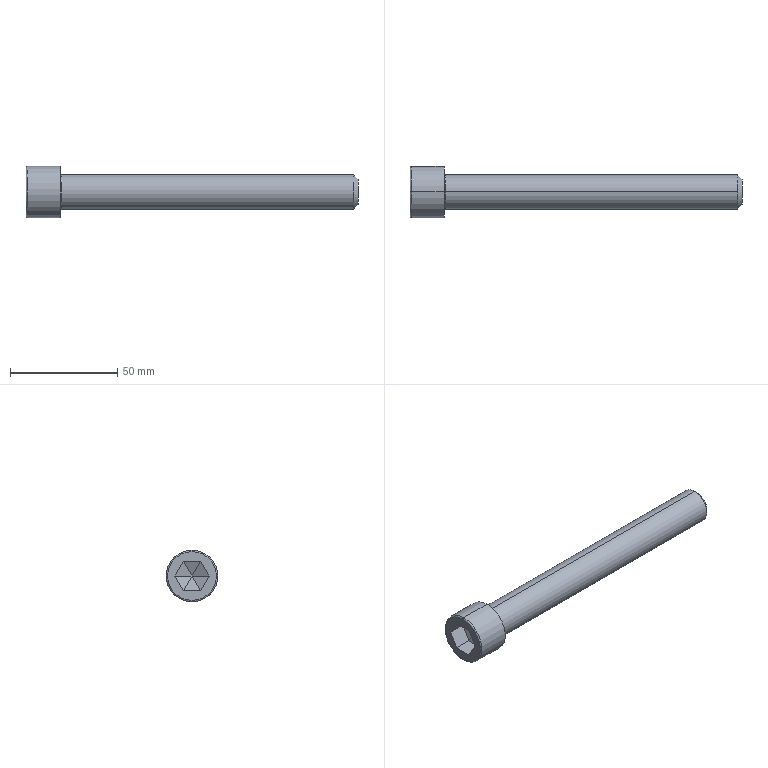Part | SolidWorks | features BlendCut 1, Chamfer 1, Cut 1, Fillet 1, ICE 1, LPattern 1, RevCut 1, Revolution 1 | 1 solid | 25 faces | box 155 x 24 x 24 mm | volume 33595 mm3 | plane 15 | torus 4 | cylinder 4 | cone 2 | commonest cylinder face diameters 16 x2 24 x2
STEP:
#1=CARTESIAN_POINT('',(155.,0.,-6.));
#2=VERTEX_POINT('',#1);
#3=CARTESIAN_POINT('',(155.,0.,6.));
#4=VERTEX_POINT('',#3);
#5=CARTESIAN_POINT('',(155.,0.,0.));
#6=DIRECTION('',(1.,0.,0.));
#7=DIRECTION('',(0.,0.,-1.));
#8=AXIS2_PLACEMENT_3D('',#5,#6,#7);
#9=CIRCLE('',#8,6.);
#10=EDGE_CURVE('',#2,#4,#9,.T.);
#11=ORIENTED_EDGE('',*,*,#10,.F.);
#12=CARTESIAN_POINT('',(153.,0.,-8.));
#13=VERTEX_POINT('',#12);
#14=CARTESIAN_POINT('',(155.,0.,-6.));
#15=DIRECTION('',(-0.7071,0.,-0.7071));
#16=VECTOR('',#15,1000.);
#17=LINE('',#14,#16);
#18=EDGE_CURVE('',#2,#13,#17,.T.);
#19=ORIENTED_EDGE('',*,*,#18,.T.);
#20=CARTESIAN_POINT('',(153.,0.,8.));
#21=VERTEX_POINT('',#20);
#22=CARTESIAN_POINT('',(153.,0.,0.));
#23=DIRECTION('',(-1.,0.,0.));
#24=DIRECTION('',(0.,0.,-1.));
#25=AXIS2_PLACEMENT_3D('',#22,#23,#24);
#26=CIRCLE('',#25,8.);
#27=EDGE_CURVE('',#21,#13,#26,.T.);
#28=ORIENTED_EDGE('',*,*,#27,.F.);
#29=CARTESIAN_POINT('',(155.,0.,6.));
#30=DIRECTION('',(-0.7071,0.,0.7071));
#31=VECTOR('',#30,1000.);
#32=LINE('',#29,#31);
#33=EDGE_CURVE('',#4,#21,#32,.T.);
#34=ORIENTED_EDGE('',*,*,#33,.F.);
#35=EDGE_LOOP('',(#11,#19,#28,#34));
#36=FACE_OUTER_BOUND('',#35,.T.);
#37=CARTESIAN_POINT('',(155.,0.,0.));
#38=DIRECTION('',(-1.,0.,0.));
#39=DIRECTION('',(0.,0.,1.));
#40=AXIS2_PLACEMENT_3D('',#37,#38,#39);
#41=CONICAL_SURFACE('',#40,6.,0.7854);
#42=ADVANCED_FACE('',(#36),#41,.T.);
#43=CARTESIAN_POINT('',(0.6,0.,-12.));
#44=VERTEX_POINT('',#43);
#45=CARTESIAN_POINT('',(0.6,0.,12.));
#46=VERTEX_POINT('',#45);
#47=CARTESIAN_POINT('',(0.6,0.,0.));
#48=DIRECTION('',(1.,0.,0.));
#49=DIRECTION('',(0.,0.,1.));
#50=AXIS2_PLACEMENT_3D('',#47,#48,#49);
#51=CIRCLE('',#50,12.);
#52=EDGE_CURVE('',#44,#46,#51,.T.);
#53=ORIENTED_EDGE('',*,*,#52,.F.);
#54=CARTESIAN_POINT('',(0.,0.,-11.4));
#55=VERTEX_POINT('',#54);
#56=CARTESIAN_POINT('',(0.6,0.,-11.4));
#57=DIRECTION('',(0.,1.,0.));
#58=DIRECTION('',(0.,0.,1.));
#59=AXIS2_PLACEMENT_3D('',#56,#57,#58);
#60=CIRCLE('',#59,0.6);
#61=EDGE_CURVE('',#44,#55,#60,.T.);
#62=ORIENTED_EDGE('',*,*,#61,.T.);
#63=CARTESIAN_POINT('',(0.,0.,11.4));
#64=VERTEX_POINT('',#63);
#65=CARTESIAN_POINT('',(0.,0.,0.));
#66=DIRECTION('',(-1.,0.,0.));
#67=DIRECTION('',(0.,0.,1.));
#68=AXIS2_PLACEMENT_3D('',#65,#66,#67);
#69=CIRCLE('',#68,11.4);
#70=EDGE_CURVE('',#64,#55,#69,.T.);
#71=ORIENTED_EDGE('',*,*,#70,.F.);
#72=CARTESIAN_POINT('',(0.6,0.,11.4));
#73=DIRECTION('',(0.,-1.,0.));
#74=DIRECTION('',(0.,0.,-1.));
#75=AXIS2_PLACEMENT_3D('',#72,#73,#74);
#76=CIRCLE('',#75,0.6);
#77=EDGE_CURVE('',#46,#64,#76,.T.);
#78=ORIENTED_EDGE('',*,*,#77,.F.);
#79=EDGE_LOOP('',(#53,#62,#71,#78));
#80=FACE_OUTER_BOUND('',#79,.T.);
#81=CARTESIAN_POINT('',(0.6,0.,0.));
#82=DIRECTION('',(-1.,0.,0.));
#83=DIRECTION('',(0.,0.,1.));
#84=AXIS2_PLACEMENT_3D('',#81,#82,#83);
#85=TOROIDAL_SURFACE('',#84,11.4,0.6);
#86=ADVANCED_FACE('',(#80),#85,.T.);
#87=CARTESIAN_POINT('',(16.6,0.,8.));
#88=VERTEX_POINT('',#87);
#89=CARTESIAN_POINT('',(16.6,0.,-8.));
#90=VERTEX_POINT('',#89);
#91=CARTESIAN_POINT('',(16.6,0.,0.));
#92=DIRECTION('',(1.,0.,0.));
#93=DIRECTION('',(0.,0.,-1.));
#94=AXIS2_PLACEMENT_3D('',#91,#92,#93);
#95=CIRCLE('',#94,8.);
#96=EDGE_CURVE('',#88,#90,#95,.T.);
#97=ORIENTED_EDGE('',*,*,#96,.F.);
#98=CARTESIAN_POINT('',(16.,0.,8.6));
#99=VERTEX_POINT('',#98);
#100=CARTESIAN_POINT('',(16.6,0.,8.6));
#101=DIRECTION('',(0.,1.,0.));
#102=DIRECTION('',(0.,0.,1.));
#103=AXIS2_PLACEMENT_3D('',#100,#101,#102);
#104=CIRCLE('',#103,0.6);
#105=EDGE_CURVE('',#88,#99,#104,.T.);
#106=ORIENTED_EDGE('',*,*,#105,.T.);
#107=CARTESIAN_POINT('',(16.,0.,-8.6));
#108=VERTEX_POINT('',#107);
#109=CARTESIAN_POINT('',(16.,0.,0.));
#110=DIRECTION('',(1.,0.,0.));
#111=DIRECTION('',(0.,0.,-1.));
#112=AXIS2_PLACEMENT_3D('',#109,#110,#111);
#113=CIRCLE('',#112,8.6);
#114=EDGE_CURVE('',#99,#108,#113,.T.);
#115=ORIENTED_EDGE('',*,*,#114,.T.);
#116=CARTESIAN_POINT('',(16.6,0.,-8.6));
#117=DIRECTION('',(0.,-1.,0.));
#118=DIRECTION('',(0.,0.,-1.));
#119=AXIS2_PLACEMENT_3D('',#116,#117,#118);
#120=CIRCLE('',#119,0.6);
#121=EDGE_CURVE('',#90,#108,#120,.T.);
#122=ORIENTED_EDGE('',*,*,#121,.F.);
#123=EDGE_LOOP('',(#97,#106,#115,#122));
#124=FACE_OUTER_BOUND('',#123,.T.);
#125=CARTESIAN_POINT('',(16.6,0.,0.));
#126=DIRECTION('',(1.,0.,0.));
#127=DIRECTION('',(0.,0.,-1.));
#128=AXIS2_PLACEMENT_3D('',#125,#126,#127);
#129=TOROIDAL_SURFACE('',#128,8.6,0.6);
#130=ADVANCED_FACE('',(#124),#129,.F.);
#131=ORIENTED_EDGE('',*,*,#52,.T.);
#132=CARTESIAN_POINT('',(16.,0.,12.));
#133=VERTEX_POINT('',#132);
#134=CARTESIAN_POINT('',(0.,0.,12.));
#135=DIRECTION('',(1.,0.,0.));
#136=VECTOR('',#135,1000.);
#137=LINE('',#134,#136);
#138=EDGE_CURVE('',#46,#133,#137,.T.);
#139=ORIENTED_EDGE('',*,*,#138,.T.);
#140=CARTESIAN_POINT('',(16.,0.,-12.));
#141=VERTEX_POINT('',#140);
#142=CARTESIAN_POINT('',(16.,0.,0.));
#143=DIRECTION('',(1.,0.,0.));
#144=DIRECTION('',(0.,0.,-1.));
#145=AXIS2_PLACEMENT_3D('',#142,#143,#144);
#146=CIRCLE('',#145,12.);
#147=EDGE_CURVE('',#141,#133,#146,.T.);
#148=ORIENTED_EDGE('',*,*,#147,.F.);
#149=CARTESIAN_POINT('',(0.,0.,-12.));
#150=DIRECTION('',(1.,0.,0.));
#151=VECTOR('',#150,1000.);
#152=LINE('',#149,#151);
#153=EDGE_CURVE('',#44,#141,#152,.T.);
#154=ORIENTED_EDGE('',*,*,#153,.F.);
#155=EDGE_LOOP('',(#131,#139,#148,#154));
#156=FACE_OUTER_BOUND('',#155,.T.);
#157=CARTESIAN_POINT('',(0.,0.,0.));
#158=DIRECTION('',(1.,0.,0.));
#159=DIRECTION('',(0.,0.,-1.));
#160=AXIS2_PLACEMENT_3D('',#157,#158,#159);
#161=CYLINDRICAL_SURFACE('',#160,12.);
#162=ADVANCED_FACE('',(#156),#161,.T.);
#163=CARTESIAN_POINT('',(16.6,0.,0.));
#164=DIRECTION('',(1.,0.,0.));
#165=DIRECTION('',(0.,0.,-1.));
#166=AXIS2_PLACEMENT_3D('',#163,#164,#165);
#167=CIRCLE('',#166,8.);
#168=EDGE_CURVE('',#90,#88,#167,.T.);
#169=ORIENTED_EDGE('',*,*,#168,.T.);
#170=CARTESIAN_POINT('',(0.,0.,8.));
#171=DIRECTION('',(1.,0.,0.));
#172=VECTOR('',#171,1000.);
#173=LINE('',#170,#172);
#174=EDGE_CURVE('',#88,#21,#173,.T.);
#175=ORIENTED_EDGE('',*,*,#174,.T.);
#176=ORIENTED_EDGE('',*,*,#27,.T.);
#177=CARTESIAN_POINT('',(0.,0.,-8.));
#178=DIRECTION('',(1.,0.,0.));
#179=VECTOR('',#178,1000.);
#180=LINE('',#177,#179);
#181=EDGE_CURVE('',#90,#13,#180,.T.);
#182=ORIENTED_EDGE('',*,*,#181,.F.);
#183=EDGE_LOOP('',(#169,#175,#176,#182));
#184=FACE_OUTER_BOUND('',#183,.T.);
#185=CARTESIAN_POINT('',(0.,0.,0.));
#186=DIRECTION('',(1.,0.,0.));
#187=DIRECTION('',(0.,0.,-1.));
#188=AXIS2_PLACEMENT_3D('',#185,#186,#187);
#189=CYLINDRICAL_SURFACE('',#188,8.);
#190=ADVANCED_FACE('',(#184),#189,.T.);
#191=ORIENTED_EDGE('',*,*,#174,.F.);
#192=ORIENTED_EDGE('',*,*,#96,.T.);
#193=ORIENTED_EDGE('',*,*,#181,.T.);
#194=CARTESIAN_POINT('',(153.,0.,0.));
#195=DIRECTION('',(-1.,0.,0.));
#196=DIRECTION('',(0.,0.,-1.));
#197=AXIS2_PLACEMENT_3D('',#194,#195,#196);
#198=CIRCLE('',#197,8.);
#199=EDGE_CURVE('',#13,#21,#198,.T.);
#200=ORIENTED_EDGE('',*,*,#199,.T.);
#201=EDGE_LOOP('',(#191,#192,#193,#200));
#202=FACE_OUTER_BOUND('',#201,.T.);
#203=CARTESIAN_POINT('',(0.,0.,0.));
#204=DIRECTION('',(1.,0.,0.));
#205=DIRECTION('',(0.,0.,-1.));
#206=AXIS2_PLACEMENT_3D('',#203,#204,#205);
#207=CYLINDRICAL_SURFACE('',#206,8.);
#208=ADVANCED_FACE('',(#202),#207,.T.);
#209=ORIENTED_EDGE('',*,*,#70,.T.);
#210=CARTESIAN_POINT('',(0.,0.,0.));
#211=DIRECTION('',(-1.,0.,0.));
#212=DIRECTION('',(0.,0.,1.));
#213=AXIS2_PLACEMENT_3D('',#210,#211,#212);
#214=CIRCLE('',#213,11.4);
#215=EDGE_CURVE('',#55,#64,#214,.T.);
#216=ORIENTED_EDGE('',*,*,#215,.T.);
#217=EDGE_LOOP('',(#209,#216));
#218=FACE_OUTER_BOUND('',#217,.T.);
#219=CARTESIAN_POINT('',(0.,-8.,0.));
#220=VERTEX_POINT('',#219);
#221=CARTESIAN_POINT('',(0.,-4.,6.928));
#222=VERTEX_POINT('',#221);
#223=CARTESIAN_POINT('',(0.,-8.,0.));
#224=DIRECTION('',(0.,0.5,0.866));
#225=VECTOR('',#224,1000.);
#226=LINE('',#223,#225);
#227=EDGE_CURVE('',#220,#222,#226,.T.);
#228=ORIENTED_EDGE('',*,*,#227,.F.);
#229=CARTESIAN_POINT('',(0.,-4.,-6.928));
#230=VERTEX_POINT('',#229);
#231=CARTESIAN_POINT('',(0.,-4.,-6.928));
#232=DIRECTION('',(0.,-0.5,0.866));
#233=VECTOR('',#232,1000.);
#234=LINE('',#231,#233);
#235=EDGE_CURVE('',#230,#220,#234,.T.);
#236=ORIENTED_EDGE('',*,*,#235,.F.);
#237=CARTESIAN_POINT('',(0.,4.,-6.928));
#238=VERTEX_POINT('',#237);
#239=CARTESIAN_POINT('',(0.,4.,-6.928));
#240=DIRECTION('',(0.,-1.,0.));
#241=VECTOR('',#240,1000.);
#242=LINE('',#239,#241);
#243=EDGE_CURVE('',#238,#230,#242,.T.);
#244=ORIENTED_EDGE('',*,*,#243,.F.);
#245=CARTESIAN_POINT('',(0.,8.,0.));
#246=VERTEX_POINT('',#245);
#247=CARTESIAN_POINT('',(0.,8.,0.));
#248=DIRECTION('',(0.,-0.5,-0.866));
#249=VECTOR('',#248,1000.);
#250=LINE('',#247,#249);
#251=EDGE_CURVE('',#246,#238,#250,.T.);
#252=ORIENTED_EDGE('',*,*,#251,.F.);
#253=CARTESIAN_POINT('',(0.,4.,6.928));
#254=VERTEX_POINT('',#253);
#255=CARTESIAN_POINT('',(0.,4.,6.928));
#256=DIRECTION('',(0.,0.5,-0.866));
#257=VECTOR('',#256,1000.);
#258=LINE('',#255,#257);
#259=EDGE_CURVE('',#254,#246,#258,.T.);
#260=ORIENTED_EDGE('',*,*,#259,.F.);
#261=CARTESIAN_POINT('',(0.,-4.,6.928));
#262=DIRECTION('',(0.,1.,0.));
#263=VECTOR('',#262,1000.);
#264=LINE('',#261,#263);
#265=EDGE_CURVE('',#222,#254,#264,.T.);
#266=ORIENTED_EDGE('',*,*,#265,.F.);
#267=EDGE_LOOP('',(#228,#236,#244,#252,#260,#266));
#268=FACE_BOUND('',#267,.T.);
#269=CARTESIAN_POINT('',(0.,0.,0.));
#270=DIRECTION('',(-1.,0.,0.));
#271=DIRECTION('',(0.,0.,1.));
#272=AXIS2_PLACEMENT_3D('',#269,#270,#271);
#273=PLANE('',#272);
#274=ADVANCED_FACE('',(#218,#268),#273,.T.);
#275=ORIENTED_EDGE('',*,*,#138,.F.);
#276=CARTESIAN_POINT('',(0.6,0.,0.));
#277=DIRECTION('',(1.,0.,0.));
#278=DIRECTION('',(0.,0.,1.));
#279=AXIS2_PLACEMENT_3D('',#276,#277,#278);
#280=CIRCLE('',#279,12.);
#281=EDGE_CURVE('',#46,#44,#280,.T.);
#282=ORIENTED_EDGE('',*,*,#281,.T.);
#283=ORIENTED_EDGE('',*,*,#153,.T.);
#284=CARTESIAN_POINT('',(16.,0.,0.));
#285=DIRECTION('',(1.,0.,0.));
#286=DIRECTION('',(0.,0.,-1.));
#287=AXIS2_PLACEMENT_3D('',#284,#285,#286);
#288=CIRCLE('',#287,12.);
#289=EDGE_CURVE('',#133,#141,#288,.T.);
#290=ORIENTED_EDGE('',*,*,#289,.F.);
#291=EDGE_LOOP('',(#275,#282,#283,#290));
#292=FACE_OUTER_BOUND('',#291,.T.);
#293=CARTESIAN_POINT('',(0.,0.,0.));
#294=DIRECTION('',(1.,0.,0.));
#295=DIRECTION('',(0.,0.,-1.));
#296=AXIS2_PLACEMENT_3D('',#293,#294,#295);
#297=CYLINDRICAL_SURFACE('',#296,12.);
#298=ADVANCED_FACE('',(#292),#297,.T.);
#299=ORIENTED_EDGE('',*,*,#147,.T.);
#300=ORIENTED_EDGE('',*,*,#289,.T.);
#301=EDGE_LOOP('',(#299,#300));
#302=FACE_OUTER_BOUND('',#301,.T.);
#303=CARTESIAN_POINT('',(16.,0.,0.));
#304=DIRECTION('',(1.,0.,0.));
#305=DIRECTION('',(0.,0.,-1.));
#306=AXIS2_PLACEMENT_3D('',#303,#304,#305);
#307=CIRCLE('',#306,8.6);
#308=EDGE_CURVE('',#108,#99,#307,.T.);
#309=ORIENTED_EDGE('',*,*,#308,.F.);
#310=ORIENTED_EDGE('',*,*,#114,.F.);
#311=EDGE_LOOP('',(#309,#310));
#312=FACE_BOUND('',#311,.T.);
#313=CARTESIAN_POINT('',(16.,12.,0.));
#314=DIRECTION('',(1.,0.,0.));
#315=DIRECTION('',(0.,0.,-1.));
#316=AXIS2_PLACEMENT_3D('',#313,#314,#315);
#317=PLANE('',#316);
#318=ADVANCED_FACE('',(#302,#312),#317,.T.);
#319=ORIENTED_EDGE('',*,*,#105,.F.);
#320=ORIENTED_EDGE('',*,*,#168,.F.);
#321=ORIENTED_EDGE('',*,*,#121,.T.);
#322=ORIENTED_EDGE('',*,*,#308,.T.);
#323=EDGE_LOOP('',(#319,#320,#321,#322));
#324=FACE_OUTER_BOUND('',#323,.T.);
#325=CARTESIAN_POINT('',(16.6,0.,0.));
#326=DIRECTION('',(1.,0.,0.));
#327=DIRECTION('',(0.,0.,-1.));
#328=AXIS2_PLACEMENT_3D('',#325,#326,#327);
#329=TOROIDAL_SURFACE('',#328,8.6,0.6);
#330=ADVANCED_FACE('',(#324),#329,.F.);
#331=ORIENTED_EDGE('',*,*,#227,.T.);
#332=CARTESIAN_POINT('',(8.,-4.,6.928));
#333=VERTEX_POINT('',#332);
#334=CARTESIAN_POINT('',(8.,-4.,6.928));
#335=DIRECTION('',(-1.,0.,0.));
#336=VECTOR('',#335,1000.);
#337=LINE('',#334,#336);
#338=EDGE_CURVE('',#333,#222,#337,.T.);
#339=ORIENTED_EDGE('',*,*,#338,.F.);
#340=CARTESIAN_POINT('',(8.,-8.,0.));
#341=VERTEX_POINT('',#340);
#342=CARTESIAN_POINT('',(8.,-8.,0.));
#343=DIRECTION('',(0.,0.5,0.866));
#344=VECTOR('',#343,1000.);
#345=LINE('',#342,#344);
#346=EDGE_CURVE('',#341,#333,#345,.T.);
#347=ORIENTED_EDGE('',*,*,#346,.F.);
#348=CARTESIAN_POINT('',(8.,-8.,0.));
#349=DIRECTION('',(-1.,0.,0.));
#350=VECTOR('',#349,1000.);
#351=LINE('',#348,#350);
#352=EDGE_CURVE('',#341,#220,#351,.T.);
#353=ORIENTED_EDGE('',*,*,#352,.T.);
#354=EDGE_LOOP('',(#331,#339,#347,#353));
#355=FACE_OUTER_BOUND('',#354,.T.);
#356=CARTESIAN_POINT('',(8.,-8.,0.));
#357=DIRECTION('',(0.,-0.866,0.5));
#358=DIRECTION('',(0.,-0.5,-0.866));
#359=AXIS2_PLACEMENT_3D('',#356,#357,#358);
#360=PLANE('',#359);
#361=ADVANCED_FACE('',(#355),#360,.F.);
#362=ORIENTED_EDGE('',*,*,#235,.T.);
#363=ORIENTED_EDGE('',*,*,#352,.F.);
#364=CARTESIAN_POINT('',(8.,-4.,-6.928));
#365=VERTEX_POINT('',#364);
#366=CARTESIAN_POINT('',(8.,-4.,-6.928));
#367=DIRECTION('',(0.,-0.5,0.866));
#368=VECTOR('',#367,1000.);
#369=LINE('',#366,#368);
#370=EDGE_CURVE('',#365,#341,#369,.T.);
#371=ORIENTED_EDGE('',*,*,#370,.F.);
#372=CARTESIAN_POINT('',(8.,-4.,-6.928));
#373=DIRECTION('',(-1.,0.,0.));
#374=VECTOR('',#373,1000.);
#375=LINE('',#372,#374);
#376=EDGE_CURVE('',#365,#230,#375,.T.);
#377=ORIENTED_EDGE('',*,*,#376,.T.);
#378=EDGE_LOOP('',(#362,#363,#371,#377));
#379=FACE_OUTER_BOUND('',#378,.T.);
#380=CARTESIAN_POINT('',(8.,-4.,-6.928));
#381=DIRECTION('',(0.,-0.866,-0.5));
#382=DIRECTION('',(0.,0.5,-0.866));
#383=AXIS2_PLACEMENT_3D('',#380,#381,#382);
#384=PLANE('',#383);
#385=ADVANCED_FACE('',(#379),#384,.F.);
#386=ORIENTED_EDGE('',*,*,#243,.T.);
#387=ORIENTED_EDGE('',*,*,#376,.F.);
#388=CARTESIAN_POINT('',(8.,4.,-6.928));
#389=VERTEX_POINT('',#388);
#390=CARTESIAN_POINT('',(8.,4.,-6.928));
#391=DIRECTION('',(0.,-1.,0.));
#392=VECTOR('',#391,1000.);
#393=LINE('',#390,#392);
#394=EDGE_CURVE('',#389,#365,#393,.T.);
#395=ORIENTED_EDGE('',*,*,#394,.F.);
#396=CARTESIAN_POINT('',(8.,4.,-6.928));
#397=DIRECTION('',(-1.,0.,0.));
#398=VECTOR('',#397,1000.);
#399=LINE('',#396,#398);
#400=EDGE_CURVE('',#389,#238,#399,.T.);
#401=ORIENTED_EDGE('',*,*,#400,.T.);
#402=EDGE_LOOP('',(#386,#387,#395,#401));
#403=FACE_OUTER_BOUND('',#402,.T.);
#404=CARTESIAN_POINT('',(8.,4.,-6.928));
#405=DIRECTION('',(0.,0.,-1.));
#406=DIRECTION('',(0.,1.,0.));
#407=AXIS2_PLACEMENT_3D('',#404,#405,#406);
#408=PLANE('',#407);
#409=ADVANCED_FACE('',(#403),#408,.F.);
#410=ORIENTED_EDGE('',*,*,#251,.T.);
#411=ORIENTED_EDGE('',*,*,#400,.F.);
#412=CARTESIAN_POINT('',(8.,8.,0.));
#413=VERTEX_POINT('',#412);
#414=CARTESIAN_POINT('',(8.,8.,0.));
#415=DIRECTION('',(0.,-0.5,-0.866));
#416=VECTOR('',#415,1000.);
#417=LINE('',#414,#416);
#418=EDGE_CURVE('',#413,#389,#417,.T.);
#419=ORIENTED_EDGE('',*,*,#418,.F.);
#420=CARTESIAN_POINT('',(8.,8.,0.));
#421=DIRECTION('',(-1.,0.,0.));
#422=VECTOR('',#421,1000.);
#423=LINE('',#420,#422);
#424=EDGE_CURVE('',#413,#246,#423,.T.);
#425=ORIENTED_EDGE('',*,*,#424,.T.);
#426=EDGE_LOOP('',(#410,#411,#419,#425));
#427=FACE_OUTER_BOUND('',#426,.T.);
#428=CARTESIAN_POINT('',(8.,8.,0.));
#429=DIRECTION('',(0.,0.866,-0.5));
#430=DIRECTION('',(0.,0.5,0.866));
#431=AXIS2_PLACEMENT_3D('',#428,#429,#430);
#432=PLANE('',#431);
#433=ADVANCED_FACE('',(#427),#432,.F.);
#434=ORIENTED_EDGE('',*,*,#259,.T.);
#435=ORIENTED_EDGE('',*,*,#424,.F.);
#436=CARTESIAN_POINT('',(8.,4.,6.928));
#437=VERTEX_POINT('',#436);
#438=CARTESIAN_POINT('',(8.,4.,6.928));
#439=DIRECTION('',(0.,0.5,-0.866));
#440=VECTOR('',#439,1000.);
#441=LINE('',#438,#440);
#442=EDGE_CURVE('',#437,#413,#441,.T.);
#443=ORIENTED_EDGE('',*,*,#442,.F.);
#444=CARTESIAN_POINT('',(8.,4.,6.928));
#445=DIRECTION('',(-1.,0.,0.));
#446=VECTOR('',#445,1000.);
#447=LINE('',#444,#446);
#448=EDGE_CURVE('',#437,#254,#447,.T.);
#449=ORIENTED_EDGE('',*,*,#448,.T.);
#450=EDGE_LOOP('',(#434,#435,#443,#449));
#451=FACE_OUTER_BOUND('',#450,.T.);
#452=CARTESIAN_POINT('',(8.,4.,6.928));
#453=DIRECTION('',(0.,0.866,0.5));
#454=DIRECTION('',(0.,-0.5,0.866));
#455=AXIS2_PLACEMENT_3D('',#452,#453,#454);
#456=PLANE('',#455);
#457=ADVANCED_FACE('',(#451),#456,.F.);
#458=ORIENTED_EDGE('',*,*,#265,.T.);
#459=ORIENTED_EDGE('',*,*,#448,.F.);
#460=CARTESIAN_POINT('',(8.,-4.,6.928));
#461=DIRECTION('',(0.,1.,0.));
#462=VECTOR('',#461,1000.);
#463=LINE('',#460,#462);
#464=EDGE_CURVE('',#333,#437,#463,.T.);
#465=ORIENTED_EDGE('',*,*,#464,.F.);
#466=ORIENTED_EDGE('',*,*,#338,.T.);
#467=EDGE_LOOP('',(#458,#459,#465,#466));
#468=FACE_OUTER_BOUND('',#467,.T.);
#469=CARTESIAN_POINT('',(8.,-4.,6.928));
#470=DIRECTION('',(0.,0.,1.));
#471=DIRECTION('',(0.,-1.,0.));
#472=AXIS2_PLACEMENT_3D('',#469,#470,#471);
#473=PLANE('',#472);
#474=ADVANCED_FACE('',(#468),#473,.F.);
#475=CARTESIAN_POINT('',(11.,0.,0.));
#476=VERTEX_POINT('',#475);
#477=CARTESIAN_POINT('',(11.,0.,0.));
#478=DIRECTION('',(-0.3511,-0.9363,0.));
#479=VECTOR('',#478,1000.);
#480=LINE('',#477,#479);
#481=EDGE_CURVE('',#476,#341,#480,.T.);
#482=ORIENTED_EDGE('',*,*,#481,.F.);
#483=CARTESIAN_POINT('',(11.,0.,0.));
#484=DIRECTION('',(-0.3511,-0.4682,-0.8109));
#485=VECTOR('',#484,1000.);
#486=LINE('',#483,#485);
#487=EDGE_CURVE('',#476,#365,#486,.T.);
#488=ORIENTED_EDGE('',*,*,#487,.T.);
#489=ORIENTED_EDGE('',*,*,#370,.T.);
#490=EDGE_LOOP('',(#482,#488,#489));
#491=FACE_OUTER_BOUND('',#490,.T.);
#492=CARTESIAN_POINT('',(8.,-8.,0.));
#493=DIRECTION('',(-0.9177,0.3441,0.1987));
#494=DIRECTION('',(-0.3511,-0.9363,0.));
#495=AXIS2_PLACEMENT_3D('',#492,#493,#494);
#496=PLANE('',#495);
#497=ADVANCED_FACE('',(#491),#496,.T.);
#498=ORIENTED_EDGE('',*,*,#487,.F.);
#499=CARTESIAN_POINT('',(11.,0.,0.));
#500=DIRECTION('',(-0.3511,0.4682,-0.8109));
#501=VECTOR('',#500,1000.);
#502=LINE('',#499,#501);
#503=EDGE_CURVE('',#476,#389,#502,.T.);
#504=ORIENTED_EDGE('',*,*,#503,.T.);
#505=ORIENTED_EDGE('',*,*,#394,.T.);
#506=EDGE_LOOP('',(#498,#504,#505));
#507=FACE_OUTER_BOUND('',#506,.T.);
#508=CARTESIAN_POINT('',(8.,-4.,-6.928));
#509=DIRECTION('',(-0.9177,0.,0.3974));
#510=DIRECTION('',(0.3974,0.,0.9177));
#511=AXIS2_PLACEMENT_3D('',#508,#509,#510);
#512=PLANE('',#511);
#513=ADVANCED_FACE('',(#507),#512,.T.);
#514=CARTESIAN_POINT('',(11.,0.,0.));
#515=DIRECTION('',(-0.3511,-0.4682,0.8109));
#516=VECTOR('',#515,1000.);
#517=LINE('',#514,#516);
#518=EDGE_CURVE('',#476,#333,#517,.T.);
#519=ORIENTED_EDGE('',*,*,#518,.F.);
#520=ORIENTED_EDGE('',*,*,#481,.T.);
#521=ORIENTED_EDGE('',*,*,#346,.T.);
#522=EDGE_LOOP('',(#519,#520,#521));
#523=FACE_OUTER_BOUND('',#522,.T.);
#524=CARTESIAN_POINT('',(8.,-4.,6.928));
#525=DIRECTION('',(-0.9177,0.3441,-0.1987));
#526=DIRECTION('',(-0.3511,-0.9363,0.));
#527=AXIS2_PLACEMENT_3D('',#524,#525,#526);
#528=PLANE('',#527);
#529=ADVANCED_FACE('',(#523),#528,.T.);
#530=ORIENTED_EDGE('',*,*,#503,.F.);
#531=CARTESIAN_POINT('',(11.,0.,0.));
#532=DIRECTION('',(-0.3511,0.9363,0.));
#533=VECTOR('',#532,1000.);
#534=LINE('',#531,#533);
#535=EDGE_CURVE('',#476,#413,#534,.T.);
#536=ORIENTED_EDGE('',*,*,#535,.T.);
#537=ORIENTED_EDGE('',*,*,#418,.T.);
#538=EDGE_LOOP('',(#530,#536,#537));
#539=FACE_OUTER_BOUND('',#538,.T.);
#540=CARTESIAN_POINT('',(8.,4.,-6.928));
#541=DIRECTION('',(-0.9177,-0.3441,0.1987));
#542=DIRECTION('',(0.3511,-0.9363,0.));
#543=AXIS2_PLACEMENT_3D('',#540,#541,#542);
#544=PLANE('',#543);
#545=ADVANCED_FACE('',(#539),#544,.T.);
#546=CARTESIAN_POINT('',(11.,0.,0.));
#547=DIRECTION('',(-0.3511,0.4682,0.8109));
#548=VECTOR('',#547,1000.);
#549=LINE('',#546,#548);
#550=EDGE_CURVE('',#476,#437,#549,.T.);
#551=ORIENTED_EDGE('',*,*,#550,.F.);
#552=ORIENTED_EDGE('',*,*,#518,.T.);
#553=ORIENTED_EDGE('',*,*,#464,.T.);
#554=EDGE_LOOP('',(#551,#552,#553));
#555=FACE_OUTER_BOUND('',#554,.T.);
#556=CARTESIAN_POINT('',(8.,4.,6.928));
#557=DIRECTION('',(-0.9177,0.,-0.3974));
#558=DIRECTION('',(-0.3974,0.,0.9177));
#559=AXIS2_PLACEMENT_3D('',#556,#557,#558);
#560=PLANE('',#559);
#561=ADVANCED_FACE('',(#555),#560,.T.);
#562=ORIENTED_EDGE('',*,*,#535,.F.);
#563=ORIENTED_EDGE('',*,*,#550,.T.);
#564=ORIENTED_EDGE('',*,*,#442,.T.);
#565=EDGE_LOOP('',(#562,#563,#564));
#566=FACE_OUTER_BOUND('',#565,.T.);
#567=CARTESIAN_POINT('',(8.,8.,0.));
#568=DIRECTION('',(-0.9177,-0.3441,-0.1987));
#569=DIRECTION('',(0.3511,-0.9363,0.));
#570=AXIS2_PLACEMENT_3D('',#567,#568,#569);
#571=PLANE('',#570);
#572=ADVANCED_FACE('',(#566),#571,.T.);
#573=ORIENTED_EDGE('',*,*,#61,.F.);
#574=ORIENTED_EDGE('',*,*,#281,.F.);
#575=ORIENTED_EDGE('',*,*,#77,.T.);
#576=ORIENTED_EDGE('',*,*,#215,.F.);
#577=EDGE_LOOP('',(#573,#574,#575,#576));
#578=FACE_OUTER_BOUND('',#577,.T.);
#579=CARTESIAN_POINT('',(0.6,0.,0.));
#580=DIRECTION('',(-1.,0.,0.));
#581=DIRECTION('',(0.,0.,1.));
#582=AXIS2_PLACEMENT_3D('',#579,#580,#581);
#583=TOROIDAL_SURFACE('',#582,11.4,0.6);
#584=ADVANCED_FACE('',(#578),#583,.T.);
#585=CARTESIAN_POINT('',(155.,0.,0.));
#586=DIRECTION('',(1.,0.,0.));
#587=DIRECTION('',(0.,0.,-1.));
#588=AXIS2_PLACEMENT_3D('',#585,#586,#587);
#589=CIRCLE('',#588,6.);
#590=EDGE_CURVE('',#4,#2,#589,.T.);
#591=ORIENTED_EDGE('',*,*,#590,.T.);
#592=ORIENTED_EDGE('',*,*,#10,.T.);
#593=EDGE_LOOP('',(#591,#592));
#594=FACE_OUTER_BOUND('',#593,.T.);
#595=CARTESIAN_POINT('',(155.,0.,0.));
#596=DIRECTION('',(1.,0.,0.));
#597=DIRECTION('',(0.,0.,-1.));
#598=AXIS2_PLACEMENT_3D('',#595,#596,#597);
#599=PLANE('',#598);
#600=ADVANCED_FACE('',(#594),#599,.T.);
#601=ORIENTED_EDGE('',*,*,#18,.F.);
#602=ORIENTED_EDGE('',*,*,#590,.F.);
#603=ORIENTED_EDGE('',*,*,#33,.T.);
#604=ORIENTED_EDGE('',*,*,#199,.F.);
#605=EDGE_LOOP('',(#601,#602,#603,#604));
#606=FACE_OUTER_BOUND('',#605,.T.);
#607=CARTESIAN_POINT('',(155.,0.,0.));
#608=DIRECTION('',(-1.,0.,0.));
#609=DIRECTION('',(0.,0.,1.));
#610=AXIS2_PLACEMENT_3D('',#607,#608,#609);
#611=CONICAL_SURFACE('',#610,6.,0.7854);
#612=ADVANCED_FACE('',(#606),#611,.T.);
#613=CLOSED_SHELL('',(#42,#86,#130,#162,#190,#208,#274,#298,#318,#330,#361,#385,#409,#433,#457,#474,#497,#513,#529,#545,#561,#572,#584,#600,#612));
#614=MANIFOLD_SOLID_BREP('',#613);
#615=CARTESIAN_POINT('',(0.,0.,0.));
#616=DIRECTION('',(0.,0.,1.));
#617=DIRECTION('',(1.,0.,0.));
#618=AXIS2_PLACEMENT_3D('',#615,#616,#617);
#619=(LENGTH_UNIT()NAMED_UNIT(*)SI_UNIT(.MILLI.,.METRE.));
#620=UNCERTAINTY_MEASURE_WITH_UNIT(LENGTH_MEASURE(0.00001),#619,'','');
#621=(NAMED_UNIT(*)PLANE_ANGLE_UNIT()SI_UNIT($,.RADIAN.));
#622=(NAMED_UNIT(*)SI_UNIT($,.STERADIAN.)SOLID_ANGLE_UNIT());
#623=(GEOMETRIC_REPRESENTATION_CONTEXT(3)GLOBAL_UNCERTAINTY_ASSIGNED_CONTEXT((#620))GLOBAL_UNIT_ASSIGNED_CONTEXT((#619,#621,#622))REPRESENTATION_CONTEXT('',''));
#624=ADVANCED_BREP_SHAPE_REPRESENTATION('',(#614,#618),#623);